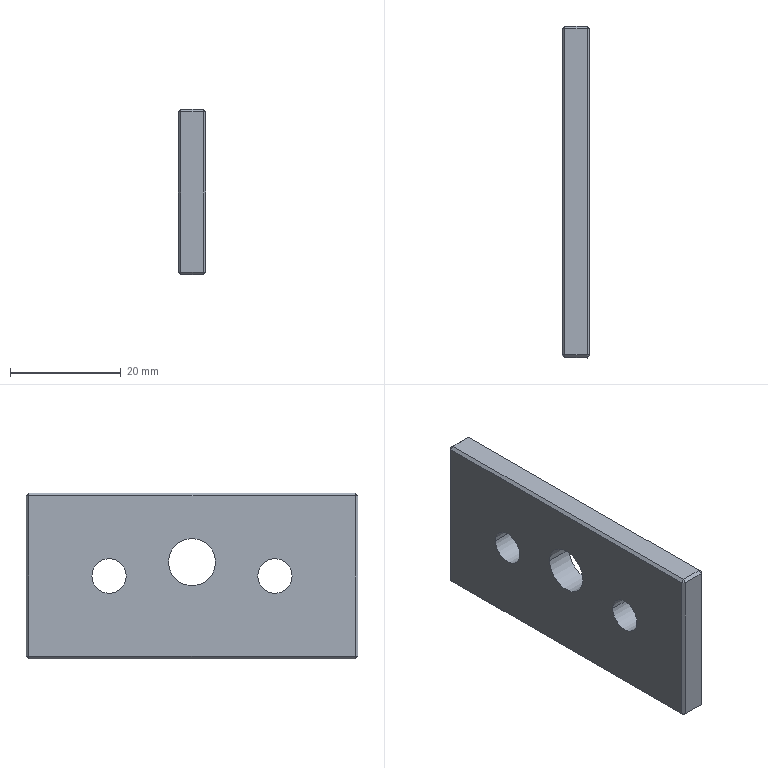Part | STEP file | 02-14 Adjusting plate | 1 solid | 32 faces | box 5 x 60 x 30 mm | volume 8368 mm3 | plane 26 | cylinder 6 | commonest cylinder face diameters 6.2 x4 8.5 x2